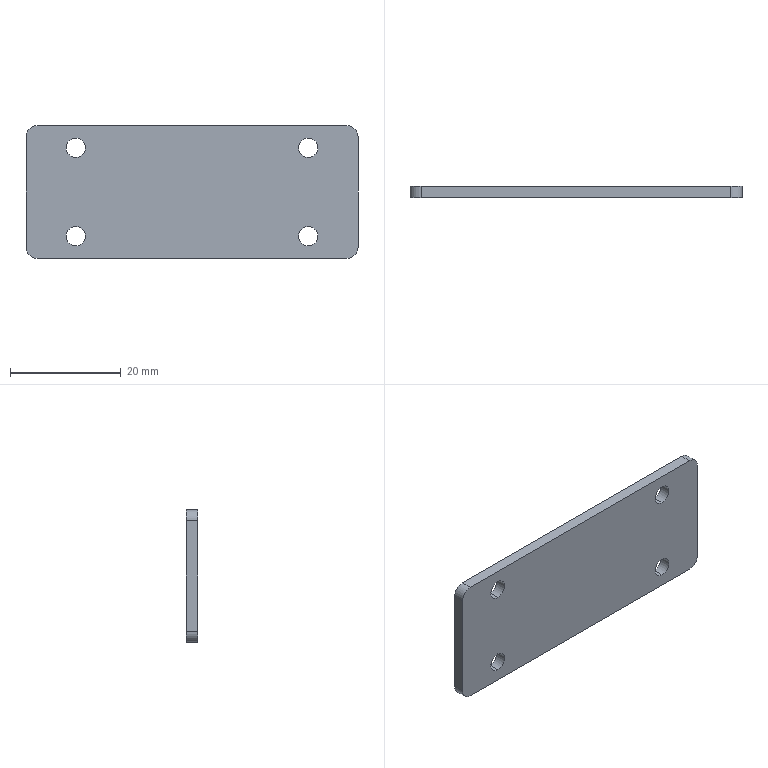Part | SolidWorks | features BaseBody 1 | 1 solid | 18 faces | box 60 x 2 x 24 mm | volume 2796 mm3 | cylinder 12 | plane 6 | commonest cylinder face diameters 3.5 x8 4 x4
STEP:
#1=CARTESIAN_POINT('',(-30.,1.,10.));
#2=VERTEX_POINT('',#1);
#3=CARTESIAN_POINT('',(-28.,1.,12.));
#4=VERTEX_POINT('',#3);
#5=CARTESIAN_POINT('',(-28.,1.,10.));
#6=DIRECTION('',(0.,1.,0.));
#7=DIRECTION('',(0.,0.,1.));
#8=AXIS2_PLACEMENT_3D('',#5,#6,#7);
#9=CIRCLE('',#8,2.);
#10=EDGE_CURVE('',#2,#4,#9,.T.);
#11=ORIENTED_EDGE('',*,*,#10,.F.);
#12=CARTESIAN_POINT('',(-30.,-1.,10.));
#13=VERTEX_POINT('',#12);
#14=CARTESIAN_POINT('',(-30.,1.,10.));
#15=DIRECTION('',(0.,1.,0.));
#16=VECTOR('',#15,1000.);
#17=LINE('',#14,#16);
#18=EDGE_CURVE('',#13,#2,#17,.T.);
#19=ORIENTED_EDGE('',*,*,#18,.F.);
#20=CARTESIAN_POINT('',(-28.,-1.,12.));
#21=VERTEX_POINT('',#20);
#22=CARTESIAN_POINT('',(-28.,-1.,10.));
#23=DIRECTION('',(0.,-1.,0.));
#24=DIRECTION('',(0.,0.,1.));
#25=AXIS2_PLACEMENT_3D('',#22,#23,#24);
#26=CIRCLE('',#25,2.);
#27=EDGE_CURVE('',#21,#13,#26,.T.);
#28=ORIENTED_EDGE('',*,*,#27,.F.);
#29=CARTESIAN_POINT('',(-28.,1.,12.));
#30=DIRECTION('',(0.,-1.,0.));
#31=VECTOR('',#30,1000.);
#32=LINE('',#29,#31);
#33=EDGE_CURVE('',#4,#21,#32,.T.);
#34=ORIENTED_EDGE('',*,*,#33,.F.);
#35=EDGE_LOOP('',(#11,#19,#28,#34));
#36=FACE_OUTER_BOUND('',#35,.T.);
#37=CARTESIAN_POINT('',(-28.,1.,10.));
#38=DIRECTION('',(0.,-1.,0.));
#39=DIRECTION('',(0.,0.,-1.));
#40=AXIS2_PLACEMENT_3D('',#37,#38,#39);
#41=CYLINDRICAL_SURFACE('',#40,2.);
#42=ADVANCED_FACE('',(#36),#41,.T.);
#43=CARTESIAN_POINT('',(-28.,1.,-12.));
#44=VERTEX_POINT('',#43);
#45=CARTESIAN_POINT('',(-30.,1.,-10.));
#46=VERTEX_POINT('',#45);
#47=CARTESIAN_POINT('',(-28.,1.,-10.));
#48=DIRECTION('',(0.,1.,0.));
#49=DIRECTION('',(0.,0.,1.));
#50=AXIS2_PLACEMENT_3D('',#47,#48,#49);
#51=CIRCLE('',#50,2.);
#52=EDGE_CURVE('',#44,#46,#51,.T.);
#53=ORIENTED_EDGE('',*,*,#52,.F.);
#54=CARTESIAN_POINT('',(-28.,-1.,-12.));
#55=VERTEX_POINT('',#54);
#56=CARTESIAN_POINT('',(-28.,1.,-12.));
#57=DIRECTION('',(0.,1.,0.));
#58=VECTOR('',#57,1000.);
#59=LINE('',#56,#58);
#60=EDGE_CURVE('',#55,#44,#59,.T.);
#61=ORIENTED_EDGE('',*,*,#60,.F.);
#62=CARTESIAN_POINT('',(-30.,-1.,-10.));
#63=VERTEX_POINT('',#62);
#64=CARTESIAN_POINT('',(-28.,-1.,-10.));
#65=DIRECTION('',(0.,-1.,0.));
#66=DIRECTION('',(0.,0.,1.));
#67=AXIS2_PLACEMENT_3D('',#64,#65,#66);
#68=CIRCLE('',#67,2.);
#69=EDGE_CURVE('',#63,#55,#68,.T.);
#70=ORIENTED_EDGE('',*,*,#69,.F.);
#71=CARTESIAN_POINT('',(-30.,1.,-10.));
#72=DIRECTION('',(0.,-1.,0.));
#73=VECTOR('',#72,1000.);
#74=LINE('',#71,#73);
#75=EDGE_CURVE('',#46,#63,#74,.T.);
#76=ORIENTED_EDGE('',*,*,#75,.F.);
#77=EDGE_LOOP('',(#53,#61,#70,#76));
#78=FACE_OUTER_BOUND('',#77,.T.);
#79=CARTESIAN_POINT('',(-28.,1.,-10.));
#80=DIRECTION('',(0.,-1.,0.));
#81=DIRECTION('',(0.,0.,-1.));
#82=AXIS2_PLACEMENT_3D('',#79,#80,#81);
#83=CYLINDRICAL_SURFACE('',#82,2.);
#84=ADVANCED_FACE('',(#78),#83,.T.);
#85=CARTESIAN_POINT('',(28.,1.,12.));
#86=VERTEX_POINT('',#85);
#87=CARTESIAN_POINT('',(30.,1.,10.));
#88=VERTEX_POINT('',#87);
#89=CARTESIAN_POINT('',(28.,1.,10.));
#90=DIRECTION('',(0.,1.,0.));
#91=DIRECTION('',(0.,0.,1.));
#92=AXIS2_PLACEMENT_3D('',#89,#90,#91);
#93=CIRCLE('',#92,2.);
#94=EDGE_CURVE('',#86,#88,#93,.T.);
#95=ORIENTED_EDGE('',*,*,#94,.F.);
#96=CARTESIAN_POINT('',(28.,-1.,12.));
#97=VERTEX_POINT('',#96);
#98=CARTESIAN_POINT('',(28.,1.,12.));
#99=DIRECTION('',(0.,1.,0.));
#100=VECTOR('',#99,1000.);
#101=LINE('',#98,#100);
#102=EDGE_CURVE('',#97,#86,#101,.T.);
#103=ORIENTED_EDGE('',*,*,#102,.F.);
#104=CARTESIAN_POINT('',(30.,-1.,10.));
#105=VERTEX_POINT('',#104);
#106=CARTESIAN_POINT('',(28.,-1.,10.));
#107=DIRECTION('',(0.,-1.,0.));
#108=DIRECTION('',(0.,0.,1.));
#109=AXIS2_PLACEMENT_3D('',#106,#107,#108);
#110=CIRCLE('',#109,2.);
#111=EDGE_CURVE('',#105,#97,#110,.T.);
#112=ORIENTED_EDGE('',*,*,#111,.F.);
#113=CARTESIAN_POINT('',(30.,1.,10.));
#114=DIRECTION('',(0.,-1.,0.));
#115=VECTOR('',#114,1000.);
#116=LINE('',#113,#115);
#117=EDGE_CURVE('',#88,#105,#116,.T.);
#118=ORIENTED_EDGE('',*,*,#117,.F.);
#119=EDGE_LOOP('',(#95,#103,#112,#118));
#120=FACE_OUTER_BOUND('',#119,.T.);
#121=CARTESIAN_POINT('',(28.,1.,10.));
#122=DIRECTION('',(0.,-1.,0.));
#123=DIRECTION('',(0.,0.,-1.));
#124=AXIS2_PLACEMENT_3D('',#121,#122,#123);
#125=CYLINDRICAL_SURFACE('',#124,2.);
#126=ADVANCED_FACE('',(#120),#125,.T.);
#127=CARTESIAN_POINT('',(30.,1.,-10.));
#128=VERTEX_POINT('',#127);
#129=CARTESIAN_POINT('',(28.,1.,-12.));
#130=VERTEX_POINT('',#129);
#131=CARTESIAN_POINT('',(28.,1.,-10.));
#132=DIRECTION('',(0.,1.,0.));
#133=DIRECTION('',(0.,0.,1.));
#134=AXIS2_PLACEMENT_3D('',#131,#132,#133);
#135=CIRCLE('',#134,2.);
#136=EDGE_CURVE('',#128,#130,#135,.T.);
#137=ORIENTED_EDGE('',*,*,#136,.F.);
#138=CARTESIAN_POINT('',(30.,-1.,-10.));
#139=VERTEX_POINT('',#138);
#140=CARTESIAN_POINT('',(30.,1.,-10.));
#141=DIRECTION('',(0.,1.,0.));
#142=VECTOR('',#141,1000.);
#143=LINE('',#140,#142);
#144=EDGE_CURVE('',#139,#128,#143,.T.);
#145=ORIENTED_EDGE('',*,*,#144,.F.);
#146=CARTESIAN_POINT('',(28.,-1.,-12.));
#147=VERTEX_POINT('',#146);
#148=CARTESIAN_POINT('',(28.,-1.,-10.));
#149=DIRECTION('',(0.,-1.,0.));
#150=DIRECTION('',(0.,0.,1.));
#151=AXIS2_PLACEMENT_3D('',#148,#149,#150);
#152=CIRCLE('',#151,2.);
#153=EDGE_CURVE('',#147,#139,#152,.T.);
#154=ORIENTED_EDGE('',*,*,#153,.F.);
#155=CARTESIAN_POINT('',(28.,1.,-12.));
#156=DIRECTION('',(0.,-1.,0.));
#157=VECTOR('',#156,1000.);
#158=LINE('',#155,#157);
#159=EDGE_CURVE('',#130,#147,#158,.T.);
#160=ORIENTED_EDGE('',*,*,#159,.F.);
#161=EDGE_LOOP('',(#137,#145,#154,#160));
#162=FACE_OUTER_BOUND('',#161,.T.);
#163=CARTESIAN_POINT('',(28.,1.,-10.));
#164=DIRECTION('',(0.,-1.,0.));
#165=DIRECTION('',(0.,0.,-1.));
#166=AXIS2_PLACEMENT_3D('',#163,#164,#165);
#167=CYLINDRICAL_SURFACE('',#166,2.);
#168=ADVANCED_FACE('',(#162),#167,.T.);
#169=CARTESIAN_POINT('',(21.,-1.,-9.75));
#170=VERTEX_POINT('',#169);
#171=CARTESIAN_POINT('',(21.,1.,-9.75));
#172=VERTEX_POINT('',#171);
#173=CARTESIAN_POINT('',(21.,-1.,-9.75));
#174=DIRECTION('',(0.,1.,0.));
#175=VECTOR('',#174,1000.);
#176=LINE('',#173,#175);
#177=EDGE_CURVE('',#170,#172,#176,.T.);
#178=ORIENTED_EDGE('',*,*,#177,.F.);
#179=CARTESIAN_POINT('',(21.,-1.,-6.25));
#180=VERTEX_POINT('',#179);
#181=CARTESIAN_POINT('',(21.,-1.,-8.));
#182=DIRECTION('',(0.,1.,0.));
#183=DIRECTION('',(0.,0.,-1.));
#184=AXIS2_PLACEMENT_3D('',#181,#182,#183);
#185=CIRCLE('',#184,1.75);
#186=EDGE_CURVE('',#180,#170,#185,.T.);
#187=ORIENTED_EDGE('',*,*,#186,.F.);
#188=CARTESIAN_POINT('',(21.,1.,-6.25));
#189=VERTEX_POINT('',#188);
#190=CARTESIAN_POINT('',(21.,-1.,-6.25));
#191=DIRECTION('',(0.,1.,0.));
#192=VECTOR('',#191,1000.);
#193=LINE('',#190,#192);
#194=EDGE_CURVE('',#180,#189,#193,.T.);
#195=ORIENTED_EDGE('',*,*,#194,.T.);
#196=CARTESIAN_POINT('',(21.,1.,-8.));
#197=DIRECTION('',(0.,1.,0.));
#198=DIRECTION('',(0.,0.,-1.));
#199=AXIS2_PLACEMENT_3D('',#196,#197,#198);
#200=CIRCLE('',#199,1.75);
#201=EDGE_CURVE('',#189,#172,#200,.T.);
#202=ORIENTED_EDGE('',*,*,#201,.T.);
#203=EDGE_LOOP('',(#178,#187,#195,#202));
#204=FACE_OUTER_BOUND('',#203,.T.);
#205=CARTESIAN_POINT('',(21.,-1.,-8.));
#206=DIRECTION('',(0.,1.,0.));
#207=DIRECTION('',(0.,0.,1.));
#208=AXIS2_PLACEMENT_3D('',#205,#206,#207);
#209=CYLINDRICAL_SURFACE('',#208,1.75);
#210=ADVANCED_FACE('',(#204),#209,.F.);
#211=CARTESIAN_POINT('',(21.,-1.,6.25));
#212=VERTEX_POINT('',#211);
#213=CARTESIAN_POINT('',(21.,1.,6.25));
#214=VERTEX_POINT('',#213);
#215=CARTESIAN_POINT('',(21.,-1.,6.25));
#216=DIRECTION('',(0.,1.,0.));
#217=VECTOR('',#216,1000.);
#218=LINE('',#215,#217);
#219=EDGE_CURVE('',#212,#214,#218,.T.);
#220=ORIENTED_EDGE('',*,*,#219,.F.);
#221=CARTESIAN_POINT('',(21.,-1.,9.75));
#222=VERTEX_POINT('',#221);
#223=CARTESIAN_POINT('',(21.,-1.,8.));
#224=DIRECTION('',(0.,1.,0.));
#225=DIRECTION('',(0.,0.,1.));
#226=AXIS2_PLACEMENT_3D('',#223,#224,#225);
#227=CIRCLE('',#226,1.75);
#228=EDGE_CURVE('',#222,#212,#227,.T.);
#229=ORIENTED_EDGE('',*,*,#228,.F.);
#230=CARTESIAN_POINT('',(21.,1.,9.75));
#231=VERTEX_POINT('',#230);
#232=CARTESIAN_POINT('',(21.,-1.,9.75));
#233=DIRECTION('',(0.,1.,0.));
#234=VECTOR('',#233,1000.);
#235=LINE('',#232,#234);
#236=EDGE_CURVE('',#222,#231,#235,.T.);
#237=ORIENTED_EDGE('',*,*,#236,.T.);
#238=CARTESIAN_POINT('',(21.,1.,8.));
#239=DIRECTION('',(0.,1.,0.));
#240=DIRECTION('',(0.,0.,1.));
#241=AXIS2_PLACEMENT_3D('',#238,#239,#240);
#242=CIRCLE('',#241,1.75);
#243=EDGE_CURVE('',#231,#214,#242,.T.);
#244=ORIENTED_EDGE('',*,*,#243,.T.);
#245=EDGE_LOOP('',(#220,#229,#237,#244));
#246=FACE_OUTER_BOUND('',#245,.T.);
#247=CARTESIAN_POINT('',(21.,-1.,8.));
#248=DIRECTION('',(0.,1.,0.));
#249=DIRECTION('',(0.,0.,1.));
#250=AXIS2_PLACEMENT_3D('',#247,#248,#249);
#251=CYLINDRICAL_SURFACE('',#250,1.75);
#252=ADVANCED_FACE('',(#246),#251,.F.);
#253=CARTESIAN_POINT('',(-21.,-1.,6.25));
#254=VERTEX_POINT('',#253);
#255=CARTESIAN_POINT('',(-21.,1.,6.25));
#256=VERTEX_POINT('',#255);
#257=CARTESIAN_POINT('',(-21.,-1.,6.25));
#258=DIRECTION('',(0.,1.,0.));
#259=VECTOR('',#258,1000.);
#260=LINE('',#257,#259);
#261=EDGE_CURVE('',#254,#256,#260,.T.);
#262=ORIENTED_EDGE('',*,*,#261,.F.);
#263=CARTESIAN_POINT('',(-21.,-1.,9.75));
#264=VERTEX_POINT('',#263);
#265=CARTESIAN_POINT('',(-21.,-1.,8.));
#266=DIRECTION('',(0.,1.,0.));
#267=DIRECTION('',(0.,0.,-1.));
#268=AXIS2_PLACEMENT_3D('',#265,#266,#267);
#269=CIRCLE('',#268,1.75);
#270=EDGE_CURVE('',#264,#254,#269,.T.);
#271=ORIENTED_EDGE('',*,*,#270,.F.);
#272=CARTESIAN_POINT('',(-21.,1.,9.75));
#273=VERTEX_POINT('',#272);
#274=CARTESIAN_POINT('',(-21.,-1.,9.75));
#275=DIRECTION('',(0.,1.,0.));
#276=VECTOR('',#275,1000.);
#277=LINE('',#274,#276);
#278=EDGE_CURVE('',#264,#273,#277,.T.);
#279=ORIENTED_EDGE('',*,*,#278,.T.);
#280=CARTESIAN_POINT('',(-21.,1.,8.));
#281=DIRECTION('',(0.,1.,0.));
#282=DIRECTION('',(0.,0.,-1.));
#283=AXIS2_PLACEMENT_3D('',#280,#281,#282);
#284=CIRCLE('',#283,1.75);
#285=EDGE_CURVE('',#273,#256,#284,.T.);
#286=ORIENTED_EDGE('',*,*,#285,.T.);
#287=EDGE_LOOP('',(#262,#271,#279,#286));
#288=FACE_OUTER_BOUND('',#287,.T.);
#289=CARTESIAN_POINT('',(-21.,-1.,8.));
#290=DIRECTION('',(0.,1.,0.));
#291=DIRECTION('',(0.,0.,1.));
#292=AXIS2_PLACEMENT_3D('',#289,#290,#291);
#293=CYLINDRICAL_SURFACE('',#292,1.75);
#294=ADVANCED_FACE('',(#288),#293,.F.);
#295=CARTESIAN_POINT('',(-21.,-1.,-9.75));
#296=VERTEX_POINT('',#295);
#297=CARTESIAN_POINT('',(-21.,1.,-9.75));
#298=VERTEX_POINT('',#297);
#299=CARTESIAN_POINT('',(-21.,-1.,-9.75));
#300=DIRECTION('',(0.,1.,0.));
#301=VECTOR('',#300,1000.);
#302=LINE('',#299,#301);
#303=EDGE_CURVE('',#296,#298,#302,.T.);
#304=ORIENTED_EDGE('',*,*,#303,.F.);
#305=CARTESIAN_POINT('',(-21.,-1.,-6.25));
#306=VERTEX_POINT('',#305);
#307=CARTESIAN_POINT('',(-21.,-1.,-8.));
#308=DIRECTION('',(0.,1.,0.));
#309=DIRECTION('',(0.,0.,1.));
#310=AXIS2_PLACEMENT_3D('',#307,#308,#309);
#311=CIRCLE('',#310,1.75);
#312=EDGE_CURVE('',#306,#296,#311,.T.);
#313=ORIENTED_EDGE('',*,*,#312,.F.);
#314=CARTESIAN_POINT('',(-21.,1.,-6.25));
#315=VERTEX_POINT('',#314);
#316=CARTESIAN_POINT('',(-21.,-1.,-6.25));
#317=DIRECTION('',(0.,1.,0.));
#318=VECTOR('',#317,1000.);
#319=LINE('',#316,#318);
#320=EDGE_CURVE('',#306,#315,#319,.T.);
#321=ORIENTED_EDGE('',*,*,#320,.T.);
#322=CARTESIAN_POINT('',(-21.,1.,-8.));
#323=DIRECTION('',(0.,1.,0.));
#324=DIRECTION('',(0.,0.,1.));
#325=AXIS2_PLACEMENT_3D('',#322,#323,#324);
#326=CIRCLE('',#325,1.75);
#327=EDGE_CURVE('',#315,#298,#326,.T.);
#328=ORIENTED_EDGE('',*,*,#327,.T.);
#329=EDGE_LOOP('',(#304,#313,#321,#328));
#330=FACE_OUTER_BOUND('',#329,.T.);
#331=CARTESIAN_POINT('',(-21.,-1.,-8.));
#332=DIRECTION('',(0.,1.,0.));
#333=DIRECTION('',(0.,0.,1.));
#334=AXIS2_PLACEMENT_3D('',#331,#332,#333);
#335=CYLINDRICAL_SURFACE('',#334,1.75);
#336=ADVANCED_FACE('',(#330),#335,.F.);
#337=ORIENTED_EDGE('',*,*,#312,.T.);
#338=CARTESIAN_POINT('',(-21.,-1.,-8.));
#339=DIRECTION('',(0.,1.,0.));
#340=DIRECTION('',(0.,0.,1.));
#341=AXIS2_PLACEMENT_3D('',#338,#339,#340);
#342=CIRCLE('',#341,1.75);
#343=EDGE_CURVE('',#296,#306,#342,.T.);
#344=ORIENTED_EDGE('',*,*,#343,.T.);
#345=EDGE_LOOP('',(#337,#344));
#346=FACE_BOUND('',#345,.T.);
#347=ORIENTED_EDGE('',*,*,#270,.T.);
#348=CARTESIAN_POINT('',(-21.,-1.,8.));
#349=DIRECTION('',(0.,1.,0.));
#350=DIRECTION('',(0.,0.,-1.));
#351=AXIS2_PLACEMENT_3D('',#348,#349,#350);
#352=CIRCLE('',#351,1.75);
#353=EDGE_CURVE('',#254,#264,#352,.T.);
#354=ORIENTED_EDGE('',*,*,#353,.T.);
#355=EDGE_LOOP('',(#347,#354));
#356=FACE_BOUND('',#355,.T.);
#357=ORIENTED_EDGE('',*,*,#228,.T.);
#358=CARTESIAN_POINT('',(21.,-1.,8.));
#359=DIRECTION('',(0.,1.,0.));
#360=DIRECTION('',(0.,0.,1.));
#361=AXIS2_PLACEMENT_3D('',#358,#359,#360);
#362=CIRCLE('',#361,1.75);
#363=EDGE_CURVE('',#212,#222,#362,.T.);
#364=ORIENTED_EDGE('',*,*,#363,.T.);
#365=EDGE_LOOP('',(#357,#364));
#366=FACE_BOUND('',#365,.T.);
#367=ORIENTED_EDGE('',*,*,#186,.T.);
#368=CARTESIAN_POINT('',(21.,-1.,-8.));
#369=DIRECTION('',(0.,1.,0.));
#370=DIRECTION('',(0.,0.,-1.));
#371=AXIS2_PLACEMENT_3D('',#368,#369,#370);
#372=CIRCLE('',#371,1.75);
#373=EDGE_CURVE('',#170,#180,#372,.T.);
#374=ORIENTED_EDGE('',*,*,#373,.T.);
#375=EDGE_LOOP('',(#367,#374));
#376=FACE_BOUND('',#375,.T.);
#377=CARTESIAN_POINT('',(-30.,-1.,-12.));
#378=DIRECTION('',(-1.,0.,0.));
#379=VECTOR('',#378,1000.);
#380=LINE('',#377,#379);
#381=EDGE_CURVE('',#147,#55,#380,.T.);
#382=ORIENTED_EDGE('',*,*,#381,.F.);
#383=ORIENTED_EDGE('',*,*,#153,.T.);
#384=CARTESIAN_POINT('',(30.,-1.,-12.));
#385=DIRECTION('',(0.,0.,-1.));
#386=VECTOR('',#385,1000.);
#387=LINE('',#384,#386);
#388=EDGE_CURVE('',#105,#139,#387,.T.);
#389=ORIENTED_EDGE('',*,*,#388,.F.);
#390=ORIENTED_EDGE('',*,*,#111,.T.);
#391=CARTESIAN_POINT('',(-30.,-1.,12.));
#392=DIRECTION('',(1.,0.,0.));
#393=VECTOR('',#392,1000.);
#394=LINE('',#391,#393);
#395=EDGE_CURVE('',#21,#97,#394,.T.);
#396=ORIENTED_EDGE('',*,*,#395,.F.);
#397=ORIENTED_EDGE('',*,*,#27,.T.);
#398=CARTESIAN_POINT('',(-30.,-1.,-12.));
#399=DIRECTION('',(0.,0.,1.));
#400=VECTOR('',#399,1000.);
#401=LINE('',#398,#400);
#402=EDGE_CURVE('',#63,#13,#401,.T.);
#403=ORIENTED_EDGE('',*,*,#402,.F.);
#404=ORIENTED_EDGE('',*,*,#69,.T.);
#405=EDGE_LOOP('',(#382,#383,#389,#390,#396,#397,#403,#404));
#406=FACE_OUTER_BOUND('',#405,.T.);
#407=CARTESIAN_POINT('',(0.,-1.,0.));
#408=DIRECTION('',(0.,1.,0.));
#409=DIRECTION('',(1.,0.,0.));
#410=AXIS2_PLACEMENT_3D('',#407,#408,#409);
#411=PLANE('',#410);
#412=ADVANCED_FACE('',(#346,#356,#366,#376,#406),#411,.F.);
#413=ORIENTED_EDGE('',*,*,#327,.F.);
#414=CARTESIAN_POINT('',(-21.,1.,-8.));
#415=DIRECTION('',(0.,1.,0.));
#416=DIRECTION('',(0.,0.,1.));
#417=AXIS2_PLACEMENT_3D('',#414,#415,#416);
#418=CIRCLE('',#417,1.75);
#419=EDGE_CURVE('',#298,#315,#418,.T.);
#420=ORIENTED_EDGE('',*,*,#419,.F.);
#421=EDGE_LOOP('',(#413,#420));
#422=FACE_BOUND('',#421,.T.);
#423=ORIENTED_EDGE('',*,*,#285,.F.);
#424=CARTESIAN_POINT('',(-21.,1.,8.));
#425=DIRECTION('',(0.,1.,0.));
#426=DIRECTION('',(0.,0.,-1.));
#427=AXIS2_PLACEMENT_3D('',#424,#425,#426);
#428=CIRCLE('',#427,1.75);
#429=EDGE_CURVE('',#256,#273,#428,.T.);
#430=ORIENTED_EDGE('',*,*,#429,.F.);
#431=EDGE_LOOP('',(#423,#430));
#432=FACE_BOUND('',#431,.T.);
#433=ORIENTED_EDGE('',*,*,#243,.F.);
#434=CARTESIAN_POINT('',(21.,1.,8.));
#435=DIRECTION('',(0.,1.,0.));
#436=DIRECTION('',(0.,0.,1.));
#437=AXIS2_PLACEMENT_3D('',#434,#435,#436);
#438=CIRCLE('',#437,1.75);
#439=EDGE_CURVE('',#214,#231,#438,.T.);
#440=ORIENTED_EDGE('',*,*,#439,.F.);
#441=EDGE_LOOP('',(#433,#440));
#442=FACE_BOUND('',#441,.T.);
#443=ORIENTED_EDGE('',*,*,#201,.F.);
#444=CARTESIAN_POINT('',(21.,1.,-8.));
#445=DIRECTION('',(0.,1.,0.));
#446=DIRECTION('',(0.,0.,-1.));
#447=AXIS2_PLACEMENT_3D('',#444,#445,#446);
#448=CIRCLE('',#447,1.75);
#449=EDGE_CURVE('',#172,#189,#448,.T.);
#450=ORIENTED_EDGE('',*,*,#449,.F.);
#451=EDGE_LOOP('',(#443,#450));
#452=FACE_BOUND('',#451,.T.);
#453=CARTESIAN_POINT('',(30.,1.,-12.));
#454=DIRECTION('',(0.,0.,-1.));
#455=VECTOR('',#454,1000.);
#456=LINE('',#453,#455);
#457=EDGE_CURVE('',#88,#128,#456,.T.);
#458=ORIENTED_EDGE('',*,*,#457,.T.);
#459=ORIENTED_EDGE('',*,*,#136,.T.);
#460=CARTESIAN_POINT('',(-30.,1.,-12.));
#461=DIRECTION('',(-1.,0.,0.));
#462=VECTOR('',#461,1000.);
#463=LINE('',#460,#462);
#464=EDGE_CURVE('',#130,#44,#463,.T.);
#465=ORIENTED_EDGE('',*,*,#464,.T.);
#466=ORIENTED_EDGE('',*,*,#52,.T.);
#467=CARTESIAN_POINT('',(-30.,1.,-12.));
#468=DIRECTION('',(0.,0.,1.));
#469=VECTOR('',#468,1000.);
#470=LINE('',#467,#469);
#471=EDGE_CURVE('',#46,#2,#470,.T.);
#472=ORIENTED_EDGE('',*,*,#471,.T.);
#473=ORIENTED_EDGE('',*,*,#10,.T.);
#474=CARTESIAN_POINT('',(-30.,1.,12.));
#475=DIRECTION('',(1.,0.,0.));
#476=VECTOR('',#475,1000.);
#477=LINE('',#474,#476);
#478=EDGE_CURVE('',#4,#86,#477,.T.);
#479=ORIENTED_EDGE('',*,*,#478,.T.);
#480=ORIENTED_EDGE('',*,*,#94,.T.);
#481=EDGE_LOOP('',(#458,#459,#465,#466,#472,#473,#479,#480));
#482=FACE_OUTER_BOUND('',#481,.T.);
#483=CARTESIAN_POINT('',(0.,1.,0.));
#484=DIRECTION('',(0.,1.,0.));
#485=DIRECTION('',(1.,0.,0.));
#486=AXIS2_PLACEMENT_3D('',#483,#484,#485);
#487=PLANE('',#486);
#488=ADVANCED_FACE('',(#422,#432,#442,#452,#482),#487,.T.);
#489=ORIENTED_EDGE('',*,*,#395,.T.);
#490=ORIENTED_EDGE('',*,*,#102,.T.);
#491=ORIENTED_EDGE('',*,*,#478,.F.);
#492=ORIENTED_EDGE('',*,*,#33,.T.);
#493=EDGE_LOOP('',(#489,#490,#491,#492));
#494=FACE_OUTER_BOUND('',#493,.T.);
#495=CARTESIAN_POINT('',(-30.,1.,12.));
#496=DIRECTION('',(0.,0.,-1.));
#497=DIRECTION('',(0.,-1.,0.));
#498=AXIS2_PLACEMENT_3D('',#495,#496,#497);
#499=PLANE('',#498);
#500=ADVANCED_FACE('',(#494),#499,.F.);
#501=ORIENTED_EDGE('',*,*,#471,.F.);
#502=ORIENTED_EDGE('',*,*,#75,.T.);
#503=ORIENTED_EDGE('',*,*,#402,.T.);
#504=ORIENTED_EDGE('',*,*,#18,.T.);
#505=EDGE_LOOP('',(#501,#502,#503,#504));
#506=FACE_OUTER_BOUND('',#505,.T.);
#507=CARTESIAN_POINT('',(-30.,1.,-12.));
#508=DIRECTION('',(1.,0.,0.));
#509=DIRECTION('',(0.,1.,0.));
#510=AXIS2_PLACEMENT_3D('',#507,#508,#509);
#511=PLANE('',#510);
#512=ADVANCED_FACE('',(#506),#511,.F.);
#513=ORIENTED_EDGE('',*,*,#464,.F.);
#514=ORIENTED_EDGE('',*,*,#159,.T.);
#515=ORIENTED_EDGE('',*,*,#381,.T.);
#516=ORIENTED_EDGE('',*,*,#60,.T.);
#517=EDGE_LOOP('',(#513,#514,#515,#516));
#518=FACE_OUTER_BOUND('',#517,.T.);
#519=CARTESIAN_POINT('',(-30.,1.,-12.));
#520=DIRECTION('',(0.,0.,1.));
#521=DIRECTION('',(1.,0.,0.));
#522=AXIS2_PLACEMENT_3D('',#519,#520,#521);
#523=PLANE('',#522);
#524=ADVANCED_FACE('',(#518),#523,.F.);
#525=ORIENTED_EDGE('',*,*,#388,.T.);
#526=ORIENTED_EDGE('',*,*,#144,.T.);
#527=ORIENTED_EDGE('',*,*,#457,.F.);
#528=ORIENTED_EDGE('',*,*,#117,.T.);
#529=EDGE_LOOP('',(#525,#526,#527,#528));
#530=FACE_OUTER_BOUND('',#529,.T.);
#531=CARTESIAN_POINT('',(30.,1.,-12.));
#532=DIRECTION('',(-1.,0.,0.));
#533=DIRECTION('',(0.,0.,1.));
#534=AXIS2_PLACEMENT_3D('',#531,#532,#533);
#535=PLANE('',#534);
#536=ADVANCED_FACE('',(#530),#535,.F.);
#537=ORIENTED_EDGE('',*,*,#343,.F.);
#538=ORIENTED_EDGE('',*,*,#303,.T.);
#539=ORIENTED_EDGE('',*,*,#419,.T.);
#540=ORIENTED_EDGE('',*,*,#320,.F.);
#541=EDGE_LOOP('',(#537,#538,#539,#540));
#542=FACE_OUTER_BOUND('',#541,.T.);
#543=CARTESIAN_POINT('',(-21.,-1.,-8.));
#544=DIRECTION('',(0.,1.,0.));
#545=DIRECTION('',(0.,0.,1.));
#546=AXIS2_PLACEMENT_3D('',#543,#544,#545);
#547=CYLINDRICAL_SURFACE('',#546,1.75);
#548=ADVANCED_FACE('',(#542),#547,.F.);
#549=ORIENTED_EDGE('',*,*,#353,.F.);
#550=ORIENTED_EDGE('',*,*,#261,.T.);
#551=ORIENTED_EDGE('',*,*,#429,.T.);
#552=ORIENTED_EDGE('',*,*,#278,.F.);
#553=EDGE_LOOP('',(#549,#550,#551,#552));
#554=FACE_OUTER_BOUND('',#553,.T.);
#555=CARTESIAN_POINT('',(-21.,-1.,8.));
#556=DIRECTION('',(0.,1.,0.));
#557=DIRECTION('',(0.,0.,1.));
#558=AXIS2_PLACEMENT_3D('',#555,#556,#557);
#559=CYLINDRICAL_SURFACE('',#558,1.75);
#560=ADVANCED_FACE('',(#554),#559,.F.);
#561=ORIENTED_EDGE('',*,*,#363,.F.);
#562=ORIENTED_EDGE('',*,*,#219,.T.);
#563=ORIENTED_EDGE('',*,*,#439,.T.);
#564=ORIENTED_EDGE('',*,*,#236,.F.);
#565=EDGE_LOOP('',(#561,#562,#563,#564));
#566=FACE_OUTER_BOUND('',#565,.T.);
#567=CARTESIAN_POINT('',(21.,-1.,8.));
#568=DIRECTION('',(0.,1.,0.));
#569=DIRECTION('',(0.,0.,1.));
#570=AXIS2_PLACEMENT_3D('',#567,#568,#569);
#571=CYLINDRICAL_SURFACE('',#570,1.75);
#572=ADVANCED_FACE('',(#566),#571,.F.);
#573=ORIENTED_EDGE('',*,*,#373,.F.);
#574=ORIENTED_EDGE('',*,*,#177,.T.);
#575=ORIENTED_EDGE('',*,*,#449,.T.);
#576=ORIENTED_EDGE('',*,*,#194,.F.);
#577=EDGE_LOOP('',(#573,#574,#575,#576));
#578=FACE_OUTER_BOUND('',#577,.T.);
#579=CARTESIAN_POINT('',(21.,-1.,-8.));
#580=DIRECTION('',(0.,1.,0.));
#581=DIRECTION('',(0.,0.,1.));
#582=AXIS2_PLACEMENT_3D('',#579,#580,#581);
#583=CYLINDRICAL_SURFACE('',#582,1.75);
#584=ADVANCED_FACE('',(#578),#583,.F.);
#585=CLOSED_SHELL('',(#42,#84,#126,#168,#210,#252,#294,#336,#412,#488,#500,#512,#524,#536,#548,#560,#572,#584));
#586=MANIFOLD_SOLID_BREP('',#585);
#587=CARTESIAN_POINT('',(0.,0.,0.));
#588=DIRECTION('',(0.,0.,1.));
#589=DIRECTION('',(1.,0.,0.));
#590=AXIS2_PLACEMENT_3D('',#587,#588,#589);
#591=(LENGTH_UNIT()NAMED_UNIT(*)SI_UNIT(.MILLI.,.METRE.));
#592=UNCERTAINTY_MEASURE_WITH_UNIT(LENGTH_MEASURE(0.00001),#591,'','');
#593=(NAMED_UNIT(*)PLANE_ANGLE_UNIT()SI_UNIT($,.RADIAN.));
#594=(NAMED_UNIT(*)SI_UNIT($,.STERADIAN.)SOLID_ANGLE_UNIT());
#595=(GEOMETRIC_REPRESENTATION_CONTEXT(3)GLOBAL_UNCERTAINTY_ASSIGNED_CONTEXT((#592))GLOBAL_UNIT_ASSIGNED_CONTEXT((#591,#593,#594))REPRESENTATION_CONTEXT('',''));
#596=ADVANCED_BREP_SHAPE_REPRESENTATION('',(#586,#590),#595);